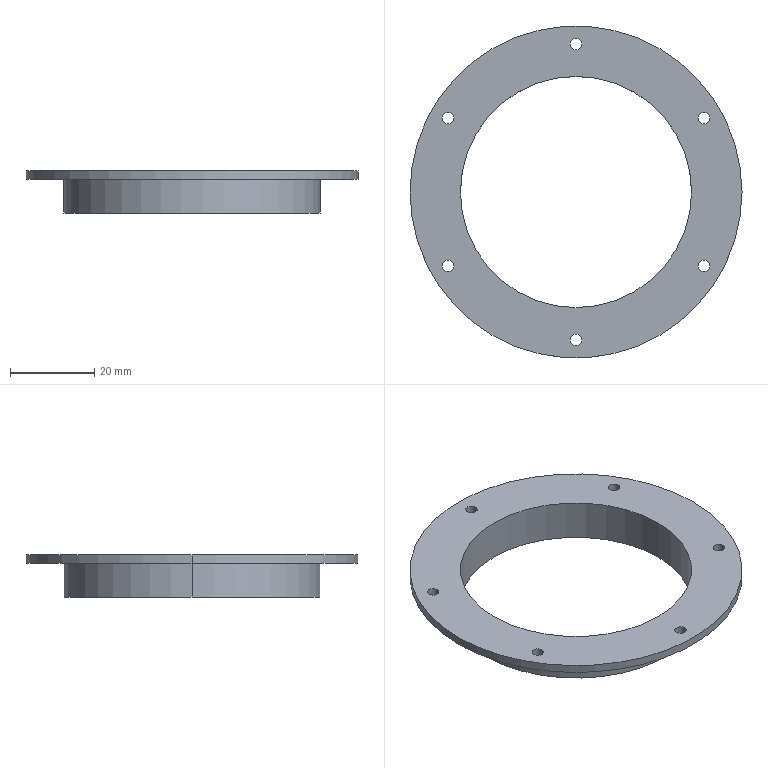Part | SolidWorks | features BaseBody 1 | 1 solid | 21 faces | box 79 x 79 x 10 mm | volume 9356 mm3 | cylinder 18 | plane 3 | commonest cylinder face diameters 2.703 x12 55 x2 61 x2 79 x2
STEP:
#1=CARTESIAN_POINT('',(27.5,0.,0.));
#2=VERTEX_POINT('',#1);
#3=CARTESIAN_POINT('',(-27.5,0.,0.));
#4=VERTEX_POINT('',#3);
#5=CARTESIAN_POINT('',(0.,0.,0.));
#6=DIRECTION('',(0.,0.,-1.));
#7=DIRECTION('',(-1.,0.,0.));
#8=AXIS2_PLACEMENT_3D('',#5,#6,#7);
#9=CIRCLE('',#8,27.5);
#10=EDGE_CURVE('',#2,#4,#9,.T.);
#11=ORIENTED_EDGE('',*,*,#10,.F.);
#12=CARTESIAN_POINT('',(27.5,0.,-10.));
#13=VERTEX_POINT('',#12);
#14=CARTESIAN_POINT('',(27.5,0.,0.));
#15=DIRECTION('',(0.,0.,-1.));
#16=VECTOR('',#15,1000.);
#17=LINE('',#14,#16);
#18=EDGE_CURVE('',#2,#13,#17,.T.);
#19=ORIENTED_EDGE('',*,*,#18,.T.);
#20=CARTESIAN_POINT('',(-27.5,0.,-10.));
#21=VERTEX_POINT('',#20);
#22=CARTESIAN_POINT('',(0.,0.,-10.));
#23=DIRECTION('',(0.,0.,1.));
#24=DIRECTION('',(-1.,0.,0.));
#25=AXIS2_PLACEMENT_3D('',#22,#23,#24);
#26=CIRCLE('',#25,27.5);
#27=EDGE_CURVE('',#21,#13,#26,.T.);
#28=ORIENTED_EDGE('',*,*,#27,.F.);
#29=CARTESIAN_POINT('',(-27.5,0.,0.));
#30=DIRECTION('',(0.,0.,-1.));
#31=VECTOR('',#30,1000.);
#32=LINE('',#29,#31);
#33=EDGE_CURVE('',#4,#21,#32,.T.);
#34=ORIENTED_EDGE('',*,*,#33,.F.);
#35=EDGE_LOOP('',(#11,#19,#28,#34));
#36=FACE_OUTER_BOUND('',#35,.T.);
#37=CARTESIAN_POINT('',(0.,0.,0.));
#38=DIRECTION('',(0.,0.,-1.));
#39=DIRECTION('',(-1.,0.,0.));
#40=AXIS2_PLACEMENT_3D('',#37,#38,#39);
#41=CYLINDRICAL_SURFACE('',#40,27.5);
#42=ADVANCED_FACE('',(#36),#41,.F.);
#43=CARTESIAN_POINT('',(-1.351,35.168,-2.));
#44=VERTEX_POINT('',#43);
#45=CARTESIAN_POINT('',(1.351,35.168,-2.));
#46=VERTEX_POINT('',#45);
#47=CARTESIAN_POINT('',(0.,35.168,-2.));
#48=DIRECTION('',(0.,0.,1.));
#49=DIRECTION('',(1.,0.,0.));
#50=AXIS2_PLACEMENT_3D('',#47,#48,#49);
#51=CIRCLE('',#50,1.351);
#52=EDGE_CURVE('',#44,#46,#51,.T.);
#53=ORIENTED_EDGE('',*,*,#52,.F.);
#54=CARTESIAN_POINT('',(-1.351,35.168,0.));
#55=VERTEX_POINT('',#54);
#56=CARTESIAN_POINT('',(-1.351,35.168,-2.));
#57=DIRECTION('',(0.,0.,1.));
#58=VECTOR('',#57,1000.);
#59=LINE('',#56,#58);
#60=EDGE_CURVE('',#44,#55,#59,.T.);
#61=ORIENTED_EDGE('',*,*,#60,.T.);
#62=CARTESIAN_POINT('',(1.351,35.168,0.));
#63=VERTEX_POINT('',#62);
#64=CARTESIAN_POINT('',(0.,35.168,0.));
#65=DIRECTION('',(0.,0.,-1.));
#66=DIRECTION('',(1.,0.,0.));
#67=AXIS2_PLACEMENT_3D('',#64,#65,#66);
#68=CIRCLE('',#67,1.351);
#69=EDGE_CURVE('',#63,#55,#68,.T.);
#70=ORIENTED_EDGE('',*,*,#69,.F.);
#71=CARTESIAN_POINT('',(1.351,35.168,-2.));
#72=DIRECTION('',(0.,0.,1.));
#73=VECTOR('',#72,1000.);
#74=LINE('',#71,#73);
#75=EDGE_CURVE('',#46,#63,#74,.T.);
#76=ORIENTED_EDGE('',*,*,#75,.F.);
#77=EDGE_LOOP('',(#53,#61,#70,#76));
#78=FACE_OUTER_BOUND('',#77,.T.);
#79=CARTESIAN_POINT('',(0.,35.168,-2.));
#80=DIRECTION('',(0.,0.,1.));
#81=DIRECTION('',(1.,0.,0.));
#82=AXIS2_PLACEMENT_3D('',#79,#80,#81);
#83=CYLINDRICAL_SURFACE('',#82,1.351);
#84=ADVANCED_FACE('',(#78),#83,.F.);
#85=CARTESIAN_POINT('',(29.105,17.584,-2.));
#86=VERTEX_POINT('',#85);
#87=CARTESIAN_POINT('',(31.807,17.584,-2.));
#88=VERTEX_POINT('',#87);
#89=CARTESIAN_POINT('',(30.456,17.584,-2.));
#90=DIRECTION('',(0.,0.,1.));
#91=DIRECTION('',(1.,0.,0.));
#92=AXIS2_PLACEMENT_3D('',#89,#90,#91);
#93=CIRCLE('',#92,1.351);
#94=EDGE_CURVE('',#86,#88,#93,.T.);
#95=ORIENTED_EDGE('',*,*,#94,.F.);
#96=CARTESIAN_POINT('',(29.105,17.584,0.));
#97=VERTEX_POINT('',#96);
#98=CARTESIAN_POINT('',(29.105,17.584,-2.));
#99=DIRECTION('',(0.,0.,1.));
#100=VECTOR('',#99,1000.);
#101=LINE('',#98,#100);
#102=EDGE_CURVE('',#86,#97,#101,.T.);
#103=ORIENTED_EDGE('',*,*,#102,.T.);
#104=CARTESIAN_POINT('',(31.807,17.584,0.));
#105=VERTEX_POINT('',#104);
#106=CARTESIAN_POINT('',(30.456,17.584,0.));
#107=DIRECTION('',(0.,0.,-1.));
#108=DIRECTION('',(1.,0.,0.));
#109=AXIS2_PLACEMENT_3D('',#106,#107,#108);
#110=CIRCLE('',#109,1.351);
#111=EDGE_CURVE('',#105,#97,#110,.T.);
#112=ORIENTED_EDGE('',*,*,#111,.F.);
#113=CARTESIAN_POINT('',(31.807,17.584,-2.));
#114=DIRECTION('',(0.,0.,1.));
#115=VECTOR('',#114,1000.);
#116=LINE('',#113,#115);
#117=EDGE_CURVE('',#88,#105,#116,.T.);
#118=ORIENTED_EDGE('',*,*,#117,.F.);
#119=EDGE_LOOP('',(#95,#103,#112,#118));
#120=FACE_OUTER_BOUND('',#119,.T.);
#121=CARTESIAN_POINT('',(30.456,17.584,-2.));
#122=DIRECTION('',(0.,0.,1.));
#123=DIRECTION('',(1.,0.,0.));
#124=AXIS2_PLACEMENT_3D('',#121,#122,#123);
#125=CYLINDRICAL_SURFACE('',#124,1.351);
#126=ADVANCED_FACE('',(#120),#125,.F.);
#127=CARTESIAN_POINT('',(29.105,-17.584,-2.));
#128=VERTEX_POINT('',#127);
#129=CARTESIAN_POINT('',(31.807,-17.584,-2.));
#130=VERTEX_POINT('',#129);
#131=CARTESIAN_POINT('',(30.456,-17.584,-2.));
#132=DIRECTION('',(0.,0.,1.));
#133=DIRECTION('',(1.,0.,0.));
#134=AXIS2_PLACEMENT_3D('',#131,#132,#133);
#135=CIRCLE('',#134,1.351);
#136=EDGE_CURVE('',#128,#130,#135,.T.);
#137=ORIENTED_EDGE('',*,*,#136,.F.);
#138=CARTESIAN_POINT('',(29.105,-17.584,0.));
#139=VERTEX_POINT('',#138);
#140=CARTESIAN_POINT('',(29.105,-17.584,-2.));
#141=DIRECTION('',(0.,0.,1.));
#142=VECTOR('',#141,1000.);
#143=LINE('',#140,#142);
#144=EDGE_CURVE('',#128,#139,#143,.T.);
#145=ORIENTED_EDGE('',*,*,#144,.T.);
#146=CARTESIAN_POINT('',(31.807,-17.584,0.));
#147=VERTEX_POINT('',#146);
#148=CARTESIAN_POINT('',(30.456,-17.584,0.));
#149=DIRECTION('',(0.,0.,-1.));
#150=DIRECTION('',(1.,0.,0.));
#151=AXIS2_PLACEMENT_3D('',#148,#149,#150);
#152=CIRCLE('',#151,1.351);
#153=EDGE_CURVE('',#147,#139,#152,.T.);
#154=ORIENTED_EDGE('',*,*,#153,.F.);
#155=CARTESIAN_POINT('',(31.807,-17.584,-2.));
#156=DIRECTION('',(0.,0.,1.));
#157=VECTOR('',#156,1000.);
#158=LINE('',#155,#157);
#159=EDGE_CURVE('',#130,#147,#158,.T.);
#160=ORIENTED_EDGE('',*,*,#159,.F.);
#161=EDGE_LOOP('',(#137,#145,#154,#160));
#162=FACE_OUTER_BOUND('',#161,.T.);
#163=CARTESIAN_POINT('',(30.456,-17.584,-2.));
#164=DIRECTION('',(0.,0.,1.));
#165=DIRECTION('',(1.,0.,0.));
#166=AXIS2_PLACEMENT_3D('',#163,#164,#165);
#167=CYLINDRICAL_SURFACE('',#166,1.351);
#168=ADVANCED_FACE('',(#162),#167,.F.);
#169=CARTESIAN_POINT('',(-1.351,-35.168,-2.));
#170=VERTEX_POINT('',#169);
#171=CARTESIAN_POINT('',(1.351,-35.168,-2.));
#172=VERTEX_POINT('',#171);
#173=CARTESIAN_POINT('',(0.,-35.168,-2.));
#174=DIRECTION('',(0.,0.,1.));
#175=DIRECTION('',(1.,0.,0.));
#176=AXIS2_PLACEMENT_3D('',#173,#174,#175);
#177=CIRCLE('',#176,1.351);
#178=EDGE_CURVE('',#170,#172,#177,.T.);
#179=ORIENTED_EDGE('',*,*,#178,.F.);
#180=CARTESIAN_POINT('',(-1.351,-35.168,0.));
#181=VERTEX_POINT('',#180);
#182=CARTESIAN_POINT('',(-1.351,-35.168,-2.));
#183=DIRECTION('',(0.,0.,1.));
#184=VECTOR('',#183,1000.);
#185=LINE('',#182,#184);
#186=EDGE_CURVE('',#170,#181,#185,.T.);
#187=ORIENTED_EDGE('',*,*,#186,.T.);
#188=CARTESIAN_POINT('',(1.351,-35.168,0.));
#189=VERTEX_POINT('',#188);
#190=CARTESIAN_POINT('',(0.,-35.168,0.));
#191=DIRECTION('',(0.,0.,-1.));
#192=DIRECTION('',(1.,0.,0.));
#193=AXIS2_PLACEMENT_3D('',#190,#191,#192);
#194=CIRCLE('',#193,1.351);
#195=EDGE_CURVE('',#189,#181,#194,.T.);
#196=ORIENTED_EDGE('',*,*,#195,.F.);
#197=CARTESIAN_POINT('',(1.351,-35.168,-2.));
#198=DIRECTION('',(0.,0.,1.));
#199=VECTOR('',#198,1000.);
#200=LINE('',#197,#199);
#201=EDGE_CURVE('',#172,#189,#200,.T.);
#202=ORIENTED_EDGE('',*,*,#201,.F.);
#203=EDGE_LOOP('',(#179,#187,#196,#202));
#204=FACE_OUTER_BOUND('',#203,.T.);
#205=CARTESIAN_POINT('',(0.,-35.168,-2.));
#206=DIRECTION('',(0.,0.,1.));
#207=DIRECTION('',(1.,0.,0.));
#208=AXIS2_PLACEMENT_3D('',#205,#206,#207);
#209=CYLINDRICAL_SURFACE('',#208,1.351);
#210=ADVANCED_FACE('',(#204),#209,.F.);
#211=CARTESIAN_POINT('',(-31.807,-17.584,-2.));
#212=VERTEX_POINT('',#211);
#213=CARTESIAN_POINT('',(-29.105,-17.584,-2.));
#214=VERTEX_POINT('',#213);
#215=CARTESIAN_POINT('',(-30.456,-17.584,-2.));
#216=DIRECTION('',(0.,0.,1.));
#217=DIRECTION('',(1.,0.,0.));
#218=AXIS2_PLACEMENT_3D('',#215,#216,#217);
#219=CIRCLE('',#218,1.351);
#220=EDGE_CURVE('',#212,#214,#219,.T.);
#221=ORIENTED_EDGE('',*,*,#220,.F.);
#222=CARTESIAN_POINT('',(-31.807,-17.584,0.));
#223=VERTEX_POINT('',#222);
#224=CARTESIAN_POINT('',(-31.807,-17.584,-2.));
#225=DIRECTION('',(0.,0.,1.));
#226=VECTOR('',#225,1000.);
#227=LINE('',#224,#226);
#228=EDGE_CURVE('',#212,#223,#227,.T.);
#229=ORIENTED_EDGE('',*,*,#228,.T.);
#230=CARTESIAN_POINT('',(-29.105,-17.584,0.));
#231=VERTEX_POINT('',#230);
#232=CARTESIAN_POINT('',(-30.456,-17.584,0.));
#233=DIRECTION('',(0.,0.,-1.));
#234=DIRECTION('',(1.,0.,0.));
#235=AXIS2_PLACEMENT_3D('',#232,#233,#234);
#236=CIRCLE('',#235,1.351);
#237=EDGE_CURVE('',#231,#223,#236,.T.);
#238=ORIENTED_EDGE('',*,*,#237,.F.);
#239=CARTESIAN_POINT('',(-29.105,-17.584,-2.));
#240=DIRECTION('',(0.,0.,1.));
#241=VECTOR('',#240,1000.);
#242=LINE('',#239,#241);
#243=EDGE_CURVE('',#214,#231,#242,.T.);
#244=ORIENTED_EDGE('',*,*,#243,.F.);
#245=EDGE_LOOP('',(#221,#229,#238,#244));
#246=FACE_OUTER_BOUND('',#245,.T.);
#247=CARTESIAN_POINT('',(-30.456,-17.584,-2.));
#248=DIRECTION('',(0.,0.,1.));
#249=DIRECTION('',(1.,0.,0.));
#250=AXIS2_PLACEMENT_3D('',#247,#248,#249);
#251=CYLINDRICAL_SURFACE('',#250,1.351);
#252=ADVANCED_FACE('',(#246),#251,.F.);
#253=CARTESIAN_POINT('',(-31.807,17.584,-2.));
#254=VERTEX_POINT('',#253);
#255=CARTESIAN_POINT('',(-29.105,17.584,-2.));
#256=VERTEX_POINT('',#255);
#257=CARTESIAN_POINT('',(-30.456,17.584,-2.));
#258=DIRECTION('',(0.,0.,1.));
#259=DIRECTION('',(1.,0.,0.));
#260=AXIS2_PLACEMENT_3D('',#257,#258,#259);
#261=CIRCLE('',#260,1.351);
#262=EDGE_CURVE('',#254,#256,#261,.T.);
#263=ORIENTED_EDGE('',*,*,#262,.F.);
#264=CARTESIAN_POINT('',(-31.807,17.584,0.));
#265=VERTEX_POINT('',#264);
#266=CARTESIAN_POINT('',(-31.807,17.584,-2.));
#267=DIRECTION('',(0.,0.,1.));
#268=VECTOR('',#267,1000.);
#269=LINE('',#266,#268);
#270=EDGE_CURVE('',#254,#265,#269,.T.);
#271=ORIENTED_EDGE('',*,*,#270,.T.);
#272=CARTESIAN_POINT('',(-29.105,17.584,0.));
#273=VERTEX_POINT('',#272);
#274=CARTESIAN_POINT('',(-30.456,17.584,0.));
#275=DIRECTION('',(0.,0.,-1.));
#276=DIRECTION('',(1.,0.,0.));
#277=AXIS2_PLACEMENT_3D('',#274,#275,#276);
#278=CIRCLE('',#277,1.351);
#279=EDGE_CURVE('',#273,#265,#278,.T.);
#280=ORIENTED_EDGE('',*,*,#279,.F.);
#281=CARTESIAN_POINT('',(-29.105,17.584,-2.));
#282=DIRECTION('',(0.,0.,1.));
#283=VECTOR('',#282,1000.);
#284=LINE('',#281,#283);
#285=EDGE_CURVE('',#256,#273,#284,.T.);
#286=ORIENTED_EDGE('',*,*,#285,.F.);
#287=EDGE_LOOP('',(#263,#271,#280,#286));
#288=FACE_OUTER_BOUND('',#287,.T.);
#289=CARTESIAN_POINT('',(-30.456,17.584,-2.));
#290=DIRECTION('',(0.,0.,1.));
#291=DIRECTION('',(1.,0.,0.));
#292=AXIS2_PLACEMENT_3D('',#289,#290,#291);
#293=CYLINDRICAL_SURFACE('',#292,1.351);
#294=ADVANCED_FACE('',(#288),#293,.F.);
#295=CARTESIAN_POINT('',(39.5,0.,0.));
#296=VERTEX_POINT('',#295);
#297=CARTESIAN_POINT('',(-39.5,0.,0.));
#298=VERTEX_POINT('',#297);
#299=CARTESIAN_POINT('',(0.,0.,0.));
#300=DIRECTION('',(0.,0.,1.));
#301=DIRECTION('',(-1.,0.,0.));
#302=AXIS2_PLACEMENT_3D('',#299,#300,#301);
#303=CIRCLE('',#302,39.5);
#304=EDGE_CURVE('',#296,#298,#303,.T.);
#305=ORIENTED_EDGE('',*,*,#304,.F.);
#306=CARTESIAN_POINT('',(39.5,0.,-2.));
#307=VERTEX_POINT('',#306);
#308=CARTESIAN_POINT('',(39.5,0.,0.));
#309=DIRECTION('',(0.,0.,-1.));
#310=VECTOR('',#309,1000.);
#311=LINE('',#308,#310);
#312=EDGE_CURVE('',#296,#307,#311,.T.);
#313=ORIENTED_EDGE('',*,*,#312,.T.);
#314=CARTESIAN_POINT('',(-39.5,0.,-2.));
#315=VERTEX_POINT('',#314);
#316=CARTESIAN_POINT('',(0.,0.,-2.));
#317=DIRECTION('',(0.,0.,1.));
#318=DIRECTION('',(-1.,0.,0.));
#319=AXIS2_PLACEMENT_3D('',#316,#317,#318);
#320=CIRCLE('',#319,39.5);
#321=EDGE_CURVE('',#307,#315,#320,.T.);
#322=ORIENTED_EDGE('',*,*,#321,.T.);
#323=CARTESIAN_POINT('',(-39.5,0.,0.));
#324=DIRECTION('',(0.,0.,-1.));
#325=VECTOR('',#324,1000.);
#326=LINE('',#323,#325);
#327=EDGE_CURVE('',#298,#315,#326,.T.);
#328=ORIENTED_EDGE('',*,*,#327,.F.);
#329=EDGE_LOOP('',(#305,#313,#322,#328));
#330=FACE_OUTER_BOUND('',#329,.T.);
#331=CARTESIAN_POINT('',(0.,0.,0.));
#332=DIRECTION('',(0.,0.,-1.));
#333=DIRECTION('',(-1.,0.,0.));
#334=AXIS2_PLACEMENT_3D('',#331,#332,#333);
#335=CYLINDRICAL_SURFACE('',#334,39.5);
#336=ADVANCED_FACE('',(#330),#335,.T.);
#337=CARTESIAN_POINT('',(-30.5,0.,-2.));
#338=VERTEX_POINT('',#337);
#339=CARTESIAN_POINT('',(30.5,0.,-2.));
#340=VERTEX_POINT('',#339);
#341=CARTESIAN_POINT('',(0.,0.,-2.));
#342=DIRECTION('',(0.,0.,-1.));
#343=DIRECTION('',(-1.,0.,0.));
#344=AXIS2_PLACEMENT_3D('',#341,#342,#343);
#345=CIRCLE('',#344,30.5);
#346=EDGE_CURVE('',#338,#340,#345,.T.);
#347=ORIENTED_EDGE('',*,*,#346,.T.);
#348=CARTESIAN_POINT('',(30.5,0.,-10.));
#349=VERTEX_POINT('',#348);
#350=CARTESIAN_POINT('',(30.5,0.,-2.));
#351=DIRECTION('',(0.,0.,-1.));
#352=VECTOR('',#351,1000.);
#353=LINE('',#350,#352);
#354=EDGE_CURVE('',#340,#349,#353,.T.);
#355=ORIENTED_EDGE('',*,*,#354,.T.);
#356=CARTESIAN_POINT('',(-30.5,0.,-10.));
#357=VERTEX_POINT('',#356);
#358=CARTESIAN_POINT('',(0.,0.,-10.));
#359=DIRECTION('',(0.,0.,-1.));
#360=DIRECTION('',(-1.,0.,0.));
#361=AXIS2_PLACEMENT_3D('',#358,#359,#360);
#362=CIRCLE('',#361,30.5);
#363=EDGE_CURVE('',#357,#349,#362,.T.);
#364=ORIENTED_EDGE('',*,*,#363,.F.);
#365=CARTESIAN_POINT('',(-30.5,0.,-2.));
#366=DIRECTION('',(0.,0.,-1.));
#367=VECTOR('',#366,1000.);
#368=LINE('',#365,#367);
#369=EDGE_CURVE('',#338,#357,#368,.T.);
#370=ORIENTED_EDGE('',*,*,#369,.F.);
#371=EDGE_LOOP('',(#347,#355,#364,#370));
#372=FACE_OUTER_BOUND('',#371,.T.);
#373=CARTESIAN_POINT('',(0.,0.,-2.));
#374=DIRECTION('',(0.,0.,-1.));
#375=DIRECTION('',(-1.,0.,0.));
#376=AXIS2_PLACEMENT_3D('',#373,#374,#375);
#377=CYLINDRICAL_SURFACE('',#376,30.5);
#378=ADVANCED_FACE('',(#372),#377,.T.);
#379=CARTESIAN_POINT('',(0.,0.,0.));
#380=DIRECTION('',(0.,0.,-1.));
#381=DIRECTION('',(-1.,0.,0.));
#382=AXIS2_PLACEMENT_3D('',#379,#380,#381);
#383=CIRCLE('',#382,27.5);
#384=EDGE_CURVE('',#4,#2,#383,.T.);
#385=ORIENTED_EDGE('',*,*,#384,.T.);
#386=ORIENTED_EDGE('',*,*,#10,.T.);
#387=EDGE_LOOP('',(#385,#386));
#388=FACE_BOUND('',#387,.T.);
#389=ORIENTED_EDGE('',*,*,#69,.T.);
#390=CARTESIAN_POINT('',(0.,35.168,0.));
#391=DIRECTION('',(0.,0.,-1.));
#392=DIRECTION('',(1.,0.,0.));
#393=AXIS2_PLACEMENT_3D('',#390,#391,#392);
#394=CIRCLE('',#393,1.351);
#395=EDGE_CURVE('',#55,#63,#394,.T.);
#396=ORIENTED_EDGE('',*,*,#395,.T.);
#397=EDGE_LOOP('',(#389,#396));
#398=FACE_BOUND('',#397,.T.);
#399=ORIENTED_EDGE('',*,*,#111,.T.);
#400=CARTESIAN_POINT('',(30.456,17.584,0.));
#401=DIRECTION('',(0.,0.,-1.));
#402=DIRECTION('',(1.,0.,0.));
#403=AXIS2_PLACEMENT_3D('',#400,#401,#402);
#404=CIRCLE('',#403,1.351);
#405=EDGE_CURVE('',#97,#105,#404,.T.);
#406=ORIENTED_EDGE('',*,*,#405,.T.);
#407=EDGE_LOOP('',(#399,#406));
#408=FACE_BOUND('',#407,.T.);
#409=ORIENTED_EDGE('',*,*,#153,.T.);
#410=CARTESIAN_POINT('',(30.456,-17.584,0.));
#411=DIRECTION('',(0.,0.,-1.));
#412=DIRECTION('',(1.,0.,0.));
#413=AXIS2_PLACEMENT_3D('',#410,#411,#412);
#414=CIRCLE('',#413,1.351);
#415=EDGE_CURVE('',#139,#147,#414,.T.);
#416=ORIENTED_EDGE('',*,*,#415,.T.);
#417=EDGE_LOOP('',(#409,#416));
#418=FACE_BOUND('',#417,.T.);
#419=ORIENTED_EDGE('',*,*,#195,.T.);
#420=CARTESIAN_POINT('',(0.,-35.168,0.));
#421=DIRECTION('',(0.,0.,-1.));
#422=DIRECTION('',(1.,0.,0.));
#423=AXIS2_PLACEMENT_3D('',#420,#421,#422);
#424=CIRCLE('',#423,1.351);
#425=EDGE_CURVE('',#181,#189,#424,.T.);
#426=ORIENTED_EDGE('',*,*,#425,.T.);
#427=EDGE_LOOP('',(#419,#426));
#428=FACE_BOUND('',#427,.T.);
#429=ORIENTED_EDGE('',*,*,#237,.T.);
#430=CARTESIAN_POINT('',(-30.456,-17.584,0.));
#431=DIRECTION('',(0.,0.,-1.));
#432=DIRECTION('',(1.,0.,0.));
#433=AXIS2_PLACEMENT_3D('',#430,#431,#432);
#434=CIRCLE('',#433,1.351);
#435=EDGE_CURVE('',#223,#231,#434,.T.);
#436=ORIENTED_EDGE('',*,*,#435,.T.);
#437=EDGE_LOOP('',(#429,#436));
#438=FACE_BOUND('',#437,.T.);
#439=ORIENTED_EDGE('',*,*,#279,.T.);
#440=CARTESIAN_POINT('',(-30.456,17.584,0.));
#441=DIRECTION('',(0.,0.,-1.));
#442=DIRECTION('',(1.,0.,0.));
#443=AXIS2_PLACEMENT_3D('',#440,#441,#442);
#444=CIRCLE('',#443,1.351);
#445=EDGE_CURVE('',#265,#273,#444,.T.);
#446=ORIENTED_EDGE('',*,*,#445,.T.);
#447=EDGE_LOOP('',(#439,#446));
#448=FACE_BOUND('',#447,.T.);
#449=CARTESIAN_POINT('',(0.,0.,0.));
#450=DIRECTION('',(0.,0.,1.));
#451=DIRECTION('',(-1.,0.,0.));
#452=AXIS2_PLACEMENT_3D('',#449,#450,#451);
#453=CIRCLE('',#452,39.5);
#454=EDGE_CURVE('',#298,#296,#453,.T.);
#455=ORIENTED_EDGE('',*,*,#454,.T.);
#456=ORIENTED_EDGE('',*,*,#304,.T.);
#457=EDGE_LOOP('',(#455,#456));
#458=FACE_OUTER_BOUND('',#457,.T.);
#459=CARTESIAN_POINT('',(0.,0.,0.));
#460=DIRECTION('',(0.,0.,1.));
#461=DIRECTION('',(1.,0.,0.));
#462=AXIS2_PLACEMENT_3D('',#459,#460,#461);
#463=PLANE('',#462);
#464=ADVANCED_FACE('',(#388,#398,#408,#418,#428,#438,#448,#458),#463,.T.);
#465=ORIENTED_EDGE('',*,*,#18,.F.);
#466=ORIENTED_EDGE('',*,*,#384,.F.);
#467=ORIENTED_EDGE('',*,*,#33,.T.);
#468=CARTESIAN_POINT('',(0.,0.,-10.));
#469=DIRECTION('',(0.,0.,1.));
#470=DIRECTION('',(-1.,0.,0.));
#471=AXIS2_PLACEMENT_3D('',#468,#469,#470);
#472=CIRCLE('',#471,27.5);
#473=EDGE_CURVE('',#13,#21,#472,.T.);
#474=ORIENTED_EDGE('',*,*,#473,.F.);
#475=EDGE_LOOP('',(#465,#466,#467,#474));
#476=FACE_OUTER_BOUND('',#475,.T.);
#477=CARTESIAN_POINT('',(0.,0.,0.));
#478=DIRECTION('',(0.,0.,-1.));
#479=DIRECTION('',(-1.,0.,0.));
#480=AXIS2_PLACEMENT_3D('',#477,#478,#479);
#481=CYLINDRICAL_SURFACE('',#480,27.5);
#482=ADVANCED_FACE('',(#476),#481,.F.);
#483=ORIENTED_EDGE('',*,*,#60,.F.);
#484=CARTESIAN_POINT('',(0.,35.168,-2.));
#485=DIRECTION('',(0.,0.,1.));
#486=DIRECTION('',(1.,0.,0.));
#487=AXIS2_PLACEMENT_3D('',#484,#485,#486);
#488=CIRCLE('',#487,1.351);
#489=EDGE_CURVE('',#46,#44,#488,.T.);
#490=ORIENTED_EDGE('',*,*,#489,.F.);
#491=ORIENTED_EDGE('',*,*,#75,.T.);
#492=ORIENTED_EDGE('',*,*,#395,.F.);
#493=EDGE_LOOP('',(#483,#490,#491,#492));
#494=FACE_OUTER_BOUND('',#493,.T.);
#495=CARTESIAN_POINT('',(0.,35.168,-2.));
#496=DIRECTION('',(0.,0.,1.));
#497=DIRECTION('',(1.,0.,0.));
#498=AXIS2_PLACEMENT_3D('',#495,#496,#497);
#499=CYLINDRICAL_SURFACE('',#498,1.351);
#500=ADVANCED_FACE('',(#494),#499,.F.);
#501=ORIENTED_EDGE('',*,*,#102,.F.);
#502=CARTESIAN_POINT('',(30.456,17.584,-2.));
#503=DIRECTION('',(0.,0.,1.));
#504=DIRECTION('',(1.,0.,0.));
#505=AXIS2_PLACEMENT_3D('',#502,#503,#504);
#506=CIRCLE('',#505,1.351);
#507=EDGE_CURVE('',#88,#86,#506,.T.);
#508=ORIENTED_EDGE('',*,*,#507,.F.);
#509=ORIENTED_EDGE('',*,*,#117,.T.);
#510=ORIENTED_EDGE('',*,*,#405,.F.);
#511=EDGE_LOOP('',(#501,#508,#509,#510));
#512=FACE_OUTER_BOUND('',#511,.T.);
#513=CARTESIAN_POINT('',(30.456,17.584,-2.));
#514=DIRECTION('',(0.,0.,1.));
#515=DIRECTION('',(1.,0.,0.));
#516=AXIS2_PLACEMENT_3D('',#513,#514,#515);
#517=CYLINDRICAL_SURFACE('',#516,1.351);
#518=ADVANCED_FACE('',(#512),#517,.F.);
#519=ORIENTED_EDGE('',*,*,#144,.F.);
#520=CARTESIAN_POINT('',(30.456,-17.584,-2.));
#521=DIRECTION('',(0.,0.,1.));
#522=DIRECTION('',(1.,0.,0.));
#523=AXIS2_PLACEMENT_3D('',#520,#521,#522);
#524=CIRCLE('',#523,1.351);
#525=EDGE_CURVE('',#130,#128,#524,.T.);
#526=ORIENTED_EDGE('',*,*,#525,.F.);
#527=ORIENTED_EDGE('',*,*,#159,.T.);
#528=ORIENTED_EDGE('',*,*,#415,.F.);
#529=EDGE_LOOP('',(#519,#526,#527,#528));
#530=FACE_OUTER_BOUND('',#529,.T.);
#531=CARTESIAN_POINT('',(30.456,-17.584,-2.));
#532=DIRECTION('',(0.,0.,1.));
#533=DIRECTION('',(1.,0.,0.));
#534=AXIS2_PLACEMENT_3D('',#531,#532,#533);
#535=CYLINDRICAL_SURFACE('',#534,1.351);
#536=ADVANCED_FACE('',(#530),#535,.F.);
#537=ORIENTED_EDGE('',*,*,#186,.F.);
#538=CARTESIAN_POINT('',(0.,-35.168,-2.));
#539=DIRECTION('',(0.,0.,1.));
#540=DIRECTION('',(1.,0.,0.));
#541=AXIS2_PLACEMENT_3D('',#538,#539,#540);
#542=CIRCLE('',#541,1.351);
#543=EDGE_CURVE('',#172,#170,#542,.T.);
#544=ORIENTED_EDGE('',*,*,#543,.F.);
#545=ORIENTED_EDGE('',*,*,#201,.T.);
#546=ORIENTED_EDGE('',*,*,#425,.F.);
#547=EDGE_LOOP('',(#537,#544,#545,#546));
#548=FACE_OUTER_BOUND('',#547,.T.);
#549=CARTESIAN_POINT('',(0.,-35.168,-2.));
#550=DIRECTION('',(0.,0.,1.));
#551=DIRECTION('',(1.,0.,0.));
#552=AXIS2_PLACEMENT_3D('',#549,#550,#551);
#553=CYLINDRICAL_SURFACE('',#552,1.351);
#554=ADVANCED_FACE('',(#548),#553,.F.);
#555=ORIENTED_EDGE('',*,*,#228,.F.);
#556=CARTESIAN_POINT('',(-30.456,-17.584,-2.));
#557=DIRECTION('',(0.,0.,1.));
#558=DIRECTION('',(1.,0.,0.));
#559=AXIS2_PLACEMENT_3D('',#556,#557,#558);
#560=CIRCLE('',#559,1.351);
#561=EDGE_CURVE('',#214,#212,#560,.T.);
#562=ORIENTED_EDGE('',*,*,#561,.F.);
#563=ORIENTED_EDGE('',*,*,#243,.T.);
#564=ORIENTED_EDGE('',*,*,#435,.F.);
#565=EDGE_LOOP('',(#555,#562,#563,#564));
#566=FACE_OUTER_BOUND('',#565,.T.);
#567=CARTESIAN_POINT('',(-30.456,-17.584,-2.));
#568=DIRECTION('',(0.,0.,1.));
#569=DIRECTION('',(1.,0.,0.));
#570=AXIS2_PLACEMENT_3D('',#567,#568,#569);
#571=CYLINDRICAL_SURFACE('',#570,1.351);
#572=ADVANCED_FACE('',(#566),#571,.F.);
#573=ORIENTED_EDGE('',*,*,#270,.F.);
#574=CARTESIAN_POINT('',(-30.456,17.584,-2.));
#575=DIRECTION('',(0.,0.,1.));
#576=DIRECTION('',(1.,0.,0.));
#577=AXIS2_PLACEMENT_3D('',#574,#575,#576);
#578=CIRCLE('',#577,1.351);
#579=EDGE_CURVE('',#256,#254,#578,.T.);
#580=ORIENTED_EDGE('',*,*,#579,.F.);
#581=ORIENTED_EDGE('',*,*,#285,.T.);
#582=ORIENTED_EDGE('',*,*,#445,.F.);
#583=EDGE_LOOP('',(#573,#580,#581,#582));
#584=FACE_OUTER_BOUND('',#583,.T.);
#585=CARTESIAN_POINT('',(-30.456,17.584,-2.));
#586=DIRECTION('',(0.,0.,1.));
#587=DIRECTION('',(1.,0.,0.));
#588=AXIS2_PLACEMENT_3D('',#585,#586,#587);
#589=CYLINDRICAL_SURFACE('',#588,1.351);
#590=ADVANCED_FACE('',(#584),#589,.F.);
#591=ORIENTED_EDGE('',*,*,#312,.F.);
#592=ORIENTED_EDGE('',*,*,#454,.F.);
#593=ORIENTED_EDGE('',*,*,#327,.T.);
#594=CARTESIAN_POINT('',(0.,0.,-2.));
#595=DIRECTION('',(0.,0.,1.));
#596=DIRECTION('',(-1.,0.,0.));
#597=AXIS2_PLACEMENT_3D('',#594,#595,#596);
#598=CIRCLE('',#597,39.5);
#599=EDGE_CURVE('',#315,#307,#598,.T.);
#600=ORIENTED_EDGE('',*,*,#599,.T.);
#601=EDGE_LOOP('',(#591,#592,#593,#600));
#602=FACE_OUTER_BOUND('',#601,.T.);
#603=CARTESIAN_POINT('',(0.,0.,0.));
#604=DIRECTION('',(0.,0.,-1.));
#605=DIRECTION('',(-1.,0.,0.));
#606=AXIS2_PLACEMENT_3D('',#603,#604,#605);
#607=CYLINDRICAL_SURFACE('',#606,39.5);
#608=ADVANCED_FACE('',(#602),#607,.T.);
#609=ORIENTED_EDGE('',*,*,#27,.T.);
#610=ORIENTED_EDGE('',*,*,#473,.T.);
#611=EDGE_LOOP('',(#609,#610));
#612=FACE_BOUND('',#611,.T.);
#613=ORIENTED_EDGE('',*,*,#363,.T.);
#614=CARTESIAN_POINT('',(0.,0.,-10.));
#615=DIRECTION('',(0.,0.,-1.));
#616=DIRECTION('',(-1.,0.,0.));
#617=AXIS2_PLACEMENT_3D('',#614,#615,#616);
#618=CIRCLE('',#617,30.5);
#619=EDGE_CURVE('',#349,#357,#618,.T.);
#620=ORIENTED_EDGE('',*,*,#619,.T.);
#621=EDGE_LOOP('',(#613,#620));
#622=FACE_OUTER_BOUND('',#621,.T.);
#623=CARTESIAN_POINT('',(0.,0.,-10.));
#624=DIRECTION('',(0.,0.,-1.));
#625=DIRECTION('',(-1.,0.,0.));
#626=AXIS2_PLACEMENT_3D('',#623,#624,#625);
#627=PLANE('',#626);
#628=ADVANCED_FACE('',(#612,#622),#627,.T.);
#629=ORIENTED_EDGE('',*,*,#346,.F.);
#630=CARTESIAN_POINT('',(0.,0.,-2.));
#631=DIRECTION('',(0.,0.,-1.));
#632=DIRECTION('',(-1.,0.,0.));
#633=AXIS2_PLACEMENT_3D('',#630,#631,#632);
#634=CIRCLE('',#633,30.5);
#635=EDGE_CURVE('',#340,#338,#634,.T.);
#636=ORIENTED_EDGE('',*,*,#635,.F.);
#637=EDGE_LOOP('',(#629,#636));
#638=FACE_BOUND('',#637,.T.);
#639=ORIENTED_EDGE('',*,*,#489,.T.);
#640=ORIENTED_EDGE('',*,*,#52,.T.);
#641=EDGE_LOOP('',(#639,#640));
#642=FACE_BOUND('',#641,.T.);
#643=ORIENTED_EDGE('',*,*,#507,.T.);
#644=ORIENTED_EDGE('',*,*,#94,.T.);
#645=EDGE_LOOP('',(#643,#644));
#646=FACE_BOUND('',#645,.T.);
#647=ORIENTED_EDGE('',*,*,#525,.T.);
#648=ORIENTED_EDGE('',*,*,#136,.T.);
#649=EDGE_LOOP('',(#647,#648));
#650=FACE_BOUND('',#649,.T.);
#651=ORIENTED_EDGE('',*,*,#543,.T.);
#652=ORIENTED_EDGE('',*,*,#178,.T.);
#653=EDGE_LOOP('',(#651,#652));
#654=FACE_BOUND('',#653,.T.);
#655=ORIENTED_EDGE('',*,*,#561,.T.);
#656=ORIENTED_EDGE('',*,*,#220,.T.);
#657=EDGE_LOOP('',(#655,#656));
#658=FACE_BOUND('',#657,.T.);
#659=ORIENTED_EDGE('',*,*,#579,.T.);
#660=ORIENTED_EDGE('',*,*,#262,.T.);
#661=EDGE_LOOP('',(#659,#660));
#662=FACE_BOUND('',#661,.T.);
#663=ORIENTED_EDGE('',*,*,#599,.F.);
#664=ORIENTED_EDGE('',*,*,#321,.F.);
#665=EDGE_LOOP('',(#663,#664));
#666=FACE_OUTER_BOUND('',#665,.T.);
#667=CARTESIAN_POINT('',(0.,0.,-2.));
#668=DIRECTION('',(0.,0.,1.));
#669=DIRECTION('',(1.,0.,0.));
#670=AXIS2_PLACEMENT_3D('',#667,#668,#669);
#671=PLANE('',#670);
#672=ADVANCED_FACE('',(#638,#642,#646,#650,#654,#658,#662,#666),#671,.F.);
#673=ORIENTED_EDGE('',*,*,#354,.F.);
#674=ORIENTED_EDGE('',*,*,#635,.T.);
#675=ORIENTED_EDGE('',*,*,#369,.T.);
#676=ORIENTED_EDGE('',*,*,#619,.F.);
#677=EDGE_LOOP('',(#673,#674,#675,#676));
#678=FACE_OUTER_BOUND('',#677,.T.);
#679=CARTESIAN_POINT('',(0.,0.,-2.));
#680=DIRECTION('',(0.,0.,-1.));
#681=DIRECTION('',(-1.,0.,0.));
#682=AXIS2_PLACEMENT_3D('',#679,#680,#681);
#683=CYLINDRICAL_SURFACE('',#682,30.5);
#684=ADVANCED_FACE('',(#678),#683,.T.);
#685=CLOSED_SHELL('',(#42,#84,#126,#168,#210,#252,#294,#336,#378,#464,#482,#500,#518,#536,#554,#572,#590,#608,#628,#672,#684));
#686=MANIFOLD_SOLID_BREP('',#685);
#687=CARTESIAN_POINT('',(0.,0.,0.));
#688=DIRECTION('',(0.,0.,1.));
#689=DIRECTION('',(1.,0.,0.));
#690=AXIS2_PLACEMENT_3D('',#687,#688,#689);
#691=(LENGTH_UNIT()NAMED_UNIT(*)SI_UNIT(.MILLI.,.METRE.));
#692=UNCERTAINTY_MEASURE_WITH_UNIT(LENGTH_MEASURE(0.00001),#691,'','');
#693=(NAMED_UNIT(*)PLANE_ANGLE_UNIT()SI_UNIT($,.RADIAN.));
#694=(NAMED_UNIT(*)SI_UNIT($,.STERADIAN.)SOLID_ANGLE_UNIT());
#695=(GEOMETRIC_REPRESENTATION_CONTEXT(3)GLOBAL_UNCERTAINTY_ASSIGNED_CONTEXT((#692))GLOBAL_UNIT_ASSIGNED_CONTEXT((#691,#693,#694))REPRESENTATION_CONTEXT('',''));
#696=ADVANCED_BREP_SHAPE_REPRESENTATION('',(#686,#690),#695);